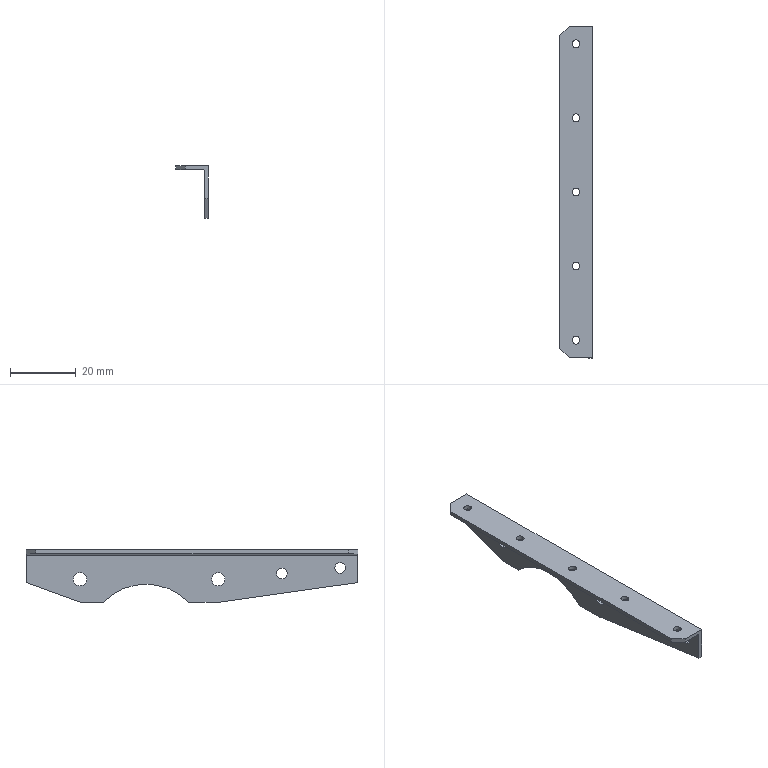Part | SolidWorks | features BaseBody 1 | 1 solid | 34 faces | box 10 x 100.8 x 16 mm | volume 2588 mm3 | cylinder 21 | plane 13 | commonest cylinder face diameters 2.4 x10 3.2 x4 4 x4 36 x2 1 x1
STEP:
#1=CARTESIAN_POINT('',(0.,5.4,-3.947));
#2=VERTEX_POINT('',#1);
#3=CARTESIAN_POINT('',(0.,5.4,-7.147));
#4=VERTEX_POINT('',#3);
#5=CARTESIAN_POINT('',(0.,5.4,-5.547));
#6=DIRECTION('',(1.,0.,0.));
#7=DIRECTION('',(0.,0.,1.));
#8=AXIS2_PLACEMENT_3D('',#5,#6,#7);
#9=CIRCLE('',#8,1.6);
#10=EDGE_CURVE('',#2,#4,#9,.T.);
#11=ORIENTED_EDGE('',*,*,#10,.T.);
#12=CARTESIAN_POINT('',(-1.2,5.4,-7.147));
#13=VERTEX_POINT('',#12);
#14=CARTESIAN_POINT('',(0.,5.4,-7.147));
#15=DIRECTION('',(-1.,0.,0.));
#16=VECTOR('',#15,1000.);
#17=LINE('',#14,#16);
#18=EDGE_CURVE('',#4,#13,#17,.T.);
#19=ORIENTED_EDGE('',*,*,#18,.T.);
#20=CARTESIAN_POINT('',(-1.2,5.4,-3.947));
#21=VERTEX_POINT('',#20);
#22=CARTESIAN_POINT('',(-1.2,5.4,-5.547));
#23=DIRECTION('',(-1.,0.,0.));
#24=DIRECTION('',(0.,0.,1.));
#25=AXIS2_PLACEMENT_3D('',#22,#23,#24);
#26=CIRCLE('',#25,1.6);
#27=EDGE_CURVE('',#13,#21,#26,.T.);
#28=ORIENTED_EDGE('',*,*,#27,.T.);
#29=CARTESIAN_POINT('',(0.,5.4,-3.947));
#30=DIRECTION('',(-1.,0.,0.));
#31=VECTOR('',#30,1000.);
#32=LINE('',#29,#31);
#33=EDGE_CURVE('',#2,#21,#32,.T.);
#34=ORIENTED_EDGE('',*,*,#33,.F.);
#35=EDGE_LOOP('',(#11,#19,#28,#34));
#36=FACE_OUTER_BOUND('',#35,.T.);
#37=CARTESIAN_POINT('',(0.,5.4,-5.547));
#38=DIRECTION('',(-1.,0.,0.));
#39=DIRECTION('',(0.,0.,1.));
#40=AXIS2_PLACEMENT_3D('',#37,#38,#39);
#41=CYLINDRICAL_SURFACE('',#40,1.6);
#42=ADVANCED_FACE('',(#36),#41,.F.);
#43=CARTESIAN_POINT('',(0.,84.4,-7.));
#44=VERTEX_POINT('',#43);
#45=CARTESIAN_POINT('',(0.,84.4,-11.));
#46=VERTEX_POINT('',#45);
#47=CARTESIAN_POINT('',(0.,84.4,-9.));
#48=DIRECTION('',(1.,0.,0.));
#49=DIRECTION('',(0.,0.,1.));
#50=AXIS2_PLACEMENT_3D('',#47,#48,#49);
#51=CIRCLE('',#50,2.);
#52=EDGE_CURVE('',#44,#46,#51,.T.);
#53=ORIENTED_EDGE('',*,*,#52,.T.);
#54=CARTESIAN_POINT('',(-1.2,84.4,-11.));
#55=VERTEX_POINT('',#54);
#56=CARTESIAN_POINT('',(0.,84.4,-11.));
#57=DIRECTION('',(-1.,0.,0.));
#58=VECTOR('',#57,1000.);
#59=LINE('',#56,#58);
#60=EDGE_CURVE('',#46,#55,#59,.T.);
#61=ORIENTED_EDGE('',*,*,#60,.T.);
#62=CARTESIAN_POINT('',(-1.2,84.4,-7.));
#63=VERTEX_POINT('',#62);
#64=CARTESIAN_POINT('',(-1.2,84.4,-9.));
#65=DIRECTION('',(-1.,0.,0.));
#66=DIRECTION('',(0.,0.,1.));
#67=AXIS2_PLACEMENT_3D('',#64,#65,#66);
#68=CIRCLE('',#67,2.);
#69=EDGE_CURVE('',#55,#63,#68,.T.);
#70=ORIENTED_EDGE('',*,*,#69,.T.);
#71=CARTESIAN_POINT('',(0.,84.4,-7.));
#72=DIRECTION('',(-1.,0.,0.));
#73=VECTOR('',#72,1000.);
#74=LINE('',#71,#73);
#75=EDGE_CURVE('',#44,#63,#74,.T.);
#76=ORIENTED_EDGE('',*,*,#75,.F.);
#77=EDGE_LOOP('',(#53,#61,#70,#76));
#78=FACE_OUTER_BOUND('',#77,.T.);
#79=CARTESIAN_POINT('',(0.,84.4,-9.));
#80=DIRECTION('',(-1.,0.,0.));
#81=DIRECTION('',(0.,0.,1.));
#82=AXIS2_PLACEMENT_3D('',#79,#80,#81);
#83=CYLINDRICAL_SURFACE('',#82,2.);
#84=ADVANCED_FACE('',(#78),#83,.F.);
#85=CARTESIAN_POINT('',(0.,42.4,-7.));
#86=VERTEX_POINT('',#85);
#87=CARTESIAN_POINT('',(0.,42.4,-11.));
#88=VERTEX_POINT('',#87);
#89=CARTESIAN_POINT('',(0.,42.4,-9.));
#90=DIRECTION('',(1.,0.,0.));
#91=DIRECTION('',(0.,0.,1.));
#92=AXIS2_PLACEMENT_3D('',#89,#90,#91);
#93=CIRCLE('',#92,2.);
#94=EDGE_CURVE('',#86,#88,#93,.T.);
#95=ORIENTED_EDGE('',*,*,#94,.T.);
#96=CARTESIAN_POINT('',(-1.2,42.4,-11.));
#97=VERTEX_POINT('',#96);
#98=CARTESIAN_POINT('',(0.,42.4,-11.));
#99=DIRECTION('',(-1.,0.,0.));
#100=VECTOR('',#99,1000.);
#101=LINE('',#98,#100);
#102=EDGE_CURVE('',#88,#97,#101,.T.);
#103=ORIENTED_EDGE('',*,*,#102,.T.);
#104=CARTESIAN_POINT('',(-1.2,42.4,-7.));
#105=VERTEX_POINT('',#104);
#106=CARTESIAN_POINT('',(-1.2,42.4,-9.));
#107=DIRECTION('',(-1.,0.,0.));
#108=DIRECTION('',(0.,0.,1.));
#109=AXIS2_PLACEMENT_3D('',#106,#107,#108);
#110=CIRCLE('',#109,2.);
#111=EDGE_CURVE('',#97,#105,#110,.T.);
#112=ORIENTED_EDGE('',*,*,#111,.T.);
#113=CARTESIAN_POINT('',(0.,42.4,-7.));
#114=DIRECTION('',(-1.,0.,0.));
#115=VECTOR('',#114,1000.);
#116=LINE('',#113,#115);
#117=EDGE_CURVE('',#86,#105,#116,.T.);
#118=ORIENTED_EDGE('',*,*,#117,.F.);
#119=EDGE_LOOP('',(#95,#103,#112,#118));
#120=FACE_OUTER_BOUND('',#119,.T.);
#121=CARTESIAN_POINT('',(0.,42.4,-9.));
#122=DIRECTION('',(-1.,0.,0.));
#123=DIRECTION('',(0.,0.,1.));
#124=AXIS2_PLACEMENT_3D('',#121,#122,#123);
#125=CYLINDRICAL_SURFACE('',#124,2.);
#126=ADVANCED_FACE('',(#120),#125,.F.);
#127=CARTESIAN_POINT('',(0.,23.103,-5.599));
#128=VERTEX_POINT('',#127);
#129=CARTESIAN_POINT('',(0.,23.103,-8.799));
#130=VERTEX_POINT('',#129);
#131=CARTESIAN_POINT('',(0.,23.103,-7.199));
#132=DIRECTION('',(1.,0.,0.));
#133=DIRECTION('',(0.,0.,1.));
#134=AXIS2_PLACEMENT_3D('',#131,#132,#133);
#135=CIRCLE('',#134,1.6);
#136=EDGE_CURVE('',#128,#130,#135,.T.);
#137=ORIENTED_EDGE('',*,*,#136,.T.);
#138=CARTESIAN_POINT('',(-1.2,23.103,-8.799));
#139=VERTEX_POINT('',#138);
#140=CARTESIAN_POINT('',(0.,23.103,-8.799));
#141=DIRECTION('',(-1.,0.,0.));
#142=VECTOR('',#141,1000.);
#143=LINE('',#140,#142);
#144=EDGE_CURVE('',#130,#139,#143,.T.);
#145=ORIENTED_EDGE('',*,*,#144,.T.);
#146=CARTESIAN_POINT('',(-1.2,23.103,-5.599));
#147=VERTEX_POINT('',#146);
#148=CARTESIAN_POINT('',(-1.2,23.103,-7.199));
#149=DIRECTION('',(-1.,0.,0.));
#150=DIRECTION('',(0.,0.,1.));
#151=AXIS2_PLACEMENT_3D('',#148,#149,#150);
#152=CIRCLE('',#151,1.6);
#153=EDGE_CURVE('',#139,#147,#152,.T.);
#154=ORIENTED_EDGE('',*,*,#153,.T.);
#155=CARTESIAN_POINT('',(0.,23.103,-5.599));
#156=DIRECTION('',(-1.,0.,0.));
#157=VECTOR('',#156,1000.);
#158=LINE('',#155,#157);
#159=EDGE_CURVE('',#128,#147,#158,.T.);
#160=ORIENTED_EDGE('',*,*,#159,.F.);
#161=EDGE_LOOP('',(#137,#145,#154,#160));
#162=FACE_OUTER_BOUND('',#161,.T.);
#163=CARTESIAN_POINT('',(0.,23.103,-7.199));
#164=DIRECTION('',(-1.,0.,0.));
#165=DIRECTION('',(0.,0.,1.));
#166=AXIS2_PLACEMENT_3D('',#163,#164,#165);
#167=CYLINDRICAL_SURFACE('',#166,1.6);
#168=ADVANCED_FACE('',(#162),#167,.F.);
#169=CARTESIAN_POINT('',(0.,77.352,-16.));
#170=VERTEX_POINT('',#169);
#171=CARTESIAN_POINT('',(0.,64.4,-10.5));
#172=VERTEX_POINT('',#171);
#173=CARTESIAN_POINT('',(0.,64.4,-28.5));
#174=DIRECTION('',(1.,0.,0.));
#175=DIRECTION('',(0.,0.,1.));
#176=AXIS2_PLACEMENT_3D('',#173,#174,#175);
#177=CIRCLE('',#176,18.);
#178=EDGE_CURVE('',#170,#172,#177,.T.);
#179=ORIENTED_EDGE('',*,*,#178,.T.);
#180=CARTESIAN_POINT('',(-1.2,64.4,-10.5));
#181=VERTEX_POINT('',#180);
#182=CARTESIAN_POINT('',(0.,64.4,-10.5));
#183=DIRECTION('',(-1.,0.,0.));
#184=VECTOR('',#183,1000.);
#185=LINE('',#182,#184);
#186=EDGE_CURVE('',#172,#181,#185,.T.);
#187=ORIENTED_EDGE('',*,*,#186,.T.);
#188=CARTESIAN_POINT('',(-1.2,77.352,-16.));
#189=VERTEX_POINT('',#188);
#190=CARTESIAN_POINT('',(-1.2,64.4,-28.5));
#191=DIRECTION('',(-1.,0.,0.));
#192=DIRECTION('',(0.,0.,1.));
#193=AXIS2_PLACEMENT_3D('',#190,#191,#192);
#194=CIRCLE('',#193,18.);
#195=EDGE_CURVE('',#181,#189,#194,.T.);
#196=ORIENTED_EDGE('',*,*,#195,.T.);
#197=CARTESIAN_POINT('',(-0.6,77.352,-16.));
#198=DIRECTION('',(1.,0.,0.));
#199=VECTOR('',#198,1000.);
#200=LINE('',#197,#199);
#201=EDGE_CURVE('',#189,#170,#200,.T.);
#202=ORIENTED_EDGE('',*,*,#201,.T.);
#203=EDGE_LOOP('',(#179,#187,#196,#202));
#204=FACE_OUTER_BOUND('',#203,.T.);
#205=CARTESIAN_POINT('',(0.,64.4,-28.5));
#206=DIRECTION('',(-1.,0.,0.));
#207=DIRECTION('',(0.,0.,1.));
#208=AXIS2_PLACEMENT_3D('',#205,#206,#207);
#209=CYLINDRICAL_SURFACE('',#208,18.);
#210=ADVANCED_FACE('',(#204),#209,.F.);
#211=CARTESIAN_POINT('',(-6.2,95.4,0.));
#212=VERTEX_POINT('',#211);
#213=CARTESIAN_POINT('',(-3.8,95.4,0.));
#214=VERTEX_POINT('',#213);
#215=CARTESIAN_POINT('',(-5.,95.4,0.));
#216=DIRECTION('',(0.,0.,1.));
#217=DIRECTION('',(-1.,0.,0.));
#218=AXIS2_PLACEMENT_3D('',#215,#216,#217);
#219=CIRCLE('',#218,1.2);
#220=EDGE_CURVE('',#212,#214,#219,.T.);
#221=ORIENTED_EDGE('',*,*,#220,.T.);
#222=CARTESIAN_POINT('',(-3.8,95.4,-1.2));
#223=VERTEX_POINT('',#222);
#224=CARTESIAN_POINT('',(-3.8,95.4,0.));
#225=DIRECTION('',(0.,0.,-1.));
#226=VECTOR('',#225,1000.);
#227=LINE('',#224,#226);
#228=EDGE_CURVE('',#214,#223,#227,.T.);
#229=ORIENTED_EDGE('',*,*,#228,.T.);
#230=CARTESIAN_POINT('',(-6.2,95.4,-1.2));
#231=VERTEX_POINT('',#230);
#232=CARTESIAN_POINT('',(-5.,95.4,-1.2));
#233=DIRECTION('',(0.,0.,-1.));
#234=DIRECTION('',(-1.,0.,0.));
#235=AXIS2_PLACEMENT_3D('',#232,#233,#234);
#236=CIRCLE('',#235,1.2);
#237=EDGE_CURVE('',#223,#231,#236,.T.);
#238=ORIENTED_EDGE('',*,*,#237,.T.);
#239=CARTESIAN_POINT('',(-6.2,95.4,0.));
#240=DIRECTION('',(0.,0.,-1.));
#241=VECTOR('',#240,1000.);
#242=LINE('',#239,#241);
#243=EDGE_CURVE('',#212,#231,#242,.T.);
#244=ORIENTED_EDGE('',*,*,#243,.F.);
#245=EDGE_LOOP('',(#221,#229,#238,#244));
#246=FACE_OUTER_BOUND('',#245,.T.);
#247=CARTESIAN_POINT('',(-5.,95.4,0.));
#248=DIRECTION('',(0.,0.,-1.));
#249=DIRECTION('',(-1.,0.,0.));
#250=AXIS2_PLACEMENT_3D('',#247,#248,#249);
#251=CYLINDRICAL_SURFACE('',#250,1.2);
#252=ADVANCED_FACE('',(#246),#251,.F.);
#253=CARTESIAN_POINT('',(-6.2,72.9,0.));
#254=VERTEX_POINT('',#253);
#255=CARTESIAN_POINT('',(-3.8,72.9,0.));
#256=VERTEX_POINT('',#255);
#257=CARTESIAN_POINT('',(-5.,72.9,0.));
#258=DIRECTION('',(0.,0.,1.));
#259=DIRECTION('',(-1.,0.,0.));
#260=AXIS2_PLACEMENT_3D('',#257,#258,#259);
#261=CIRCLE('',#260,1.2);
#262=EDGE_CURVE('',#254,#256,#261,.T.);
#263=ORIENTED_EDGE('',*,*,#262,.T.);
#264=CARTESIAN_POINT('',(-3.8,72.9,-1.2));
#265=VERTEX_POINT('',#264);
#266=CARTESIAN_POINT('',(-3.8,72.9,0.));
#267=DIRECTION('',(0.,0.,-1.));
#268=VECTOR('',#267,1000.);
#269=LINE('',#266,#268);
#270=EDGE_CURVE('',#256,#265,#269,.T.);
#271=ORIENTED_EDGE('',*,*,#270,.T.);
#272=CARTESIAN_POINT('',(-6.2,72.9,-1.2));
#273=VERTEX_POINT('',#272);
#274=CARTESIAN_POINT('',(-5.,72.9,-1.2));
#275=DIRECTION('',(0.,0.,-1.));
#276=DIRECTION('',(-1.,0.,0.));
#277=AXIS2_PLACEMENT_3D('',#274,#275,#276);
#278=CIRCLE('',#277,1.2);
#279=EDGE_CURVE('',#265,#273,#278,.T.);
#280=ORIENTED_EDGE('',*,*,#279,.T.);
#281=CARTESIAN_POINT('',(-6.2,72.9,0.));
#282=DIRECTION('',(0.,0.,-1.));
#283=VECTOR('',#282,1000.);
#284=LINE('',#281,#283);
#285=EDGE_CURVE('',#254,#273,#284,.T.);
#286=ORIENTED_EDGE('',*,*,#285,.F.);
#287=EDGE_LOOP('',(#263,#271,#280,#286));
#288=FACE_OUTER_BOUND('',#287,.T.);
#289=CARTESIAN_POINT('',(-5.,72.9,0.));
#290=DIRECTION('',(0.,0.,-1.));
#291=DIRECTION('',(-1.,0.,0.));
#292=AXIS2_PLACEMENT_3D('',#289,#290,#291);
#293=CYLINDRICAL_SURFACE('',#292,1.2);
#294=ADVANCED_FACE('',(#288),#293,.F.);
#295=CARTESIAN_POINT('',(-6.2,50.4,0.));
#296=VERTEX_POINT('',#295);
#297=CARTESIAN_POINT('',(-3.8,50.4,0.));
#298=VERTEX_POINT('',#297);
#299=CARTESIAN_POINT('',(-5.,50.4,0.));
#300=DIRECTION('',(0.,0.,1.));
#301=DIRECTION('',(-1.,0.,0.));
#302=AXIS2_PLACEMENT_3D('',#299,#300,#301);
#303=CIRCLE('',#302,1.2);
#304=EDGE_CURVE('',#296,#298,#303,.T.);
#305=ORIENTED_EDGE('',*,*,#304,.T.);
#306=CARTESIAN_POINT('',(-3.8,50.4,-1.2));
#307=VERTEX_POINT('',#306);
#308=CARTESIAN_POINT('',(-3.8,50.4,0.));
#309=DIRECTION('',(0.,0.,-1.));
#310=VECTOR('',#309,1000.);
#311=LINE('',#308,#310);
#312=EDGE_CURVE('',#298,#307,#311,.T.);
#313=ORIENTED_EDGE('',*,*,#312,.T.);
#314=CARTESIAN_POINT('',(-6.2,50.4,-1.2));
#315=VERTEX_POINT('',#314);
#316=CARTESIAN_POINT('',(-5.,50.4,-1.2));
#317=DIRECTION('',(0.,0.,-1.));
#318=DIRECTION('',(-1.,0.,0.));
#319=AXIS2_PLACEMENT_3D('',#316,#317,#318);
#320=CIRCLE('',#319,1.2);
#321=EDGE_CURVE('',#307,#315,#320,.T.);
#322=ORIENTED_EDGE('',*,*,#321,.T.);
#323=CARTESIAN_POINT('',(-6.2,50.4,0.));
#324=DIRECTION('',(0.,0.,-1.));
#325=VECTOR('',#324,1000.);
#326=LINE('',#323,#325);
#327=EDGE_CURVE('',#296,#315,#326,.T.);
#328=ORIENTED_EDGE('',*,*,#327,.F.);
#329=EDGE_LOOP('',(#305,#313,#322,#328));
#330=FACE_OUTER_BOUND('',#329,.T.);
#331=CARTESIAN_POINT('',(-5.,50.4,0.));
#332=DIRECTION('',(0.,0.,-1.));
#333=DIRECTION('',(-1.,0.,0.));
#334=AXIS2_PLACEMENT_3D('',#331,#332,#333);
#335=CYLINDRICAL_SURFACE('',#334,1.2);
#336=ADVANCED_FACE('',(#330),#335,.F.);
#337=CARTESIAN_POINT('',(-6.2,5.4,0.));
#338=VERTEX_POINT('',#337);
#339=CARTESIAN_POINT('',(-3.8,5.4,0.));
#340=VERTEX_POINT('',#339);
#341=CARTESIAN_POINT('',(-5.,5.4,0.));
#342=DIRECTION('',(0.,0.,1.));
#343=DIRECTION('',(-1.,0.,0.));
#344=AXIS2_PLACEMENT_3D('',#341,#342,#343);
#345=CIRCLE('',#344,1.2);
#346=EDGE_CURVE('',#338,#340,#345,.T.);
#347=ORIENTED_EDGE('',*,*,#346,.T.);
#348=CARTESIAN_POINT('',(-3.8,5.4,-1.2));
#349=VERTEX_POINT('',#348);
#350=CARTESIAN_POINT('',(-3.8,5.4,0.));
#351=DIRECTION('',(0.,0.,-1.));
#352=VECTOR('',#351,1000.);
#353=LINE('',#350,#352);
#354=EDGE_CURVE('',#340,#349,#353,.T.);
#355=ORIENTED_EDGE('',*,*,#354,.T.);
#356=CARTESIAN_POINT('',(-6.2,5.4,-1.2));
#357=VERTEX_POINT('',#356);
#358=CARTESIAN_POINT('',(-5.,5.4,-1.2));
#359=DIRECTION('',(0.,0.,-1.));
#360=DIRECTION('',(-1.,0.,0.));
#361=AXIS2_PLACEMENT_3D('',#358,#359,#360);
#362=CIRCLE('',#361,1.2);
#363=EDGE_CURVE('',#349,#357,#362,.T.);
#364=ORIENTED_EDGE('',*,*,#363,.T.);
#365=CARTESIAN_POINT('',(-6.2,5.4,0.));
#366=DIRECTION('',(0.,0.,-1.));
#367=VECTOR('',#366,1000.);
#368=LINE('',#365,#367);
#369=EDGE_CURVE('',#338,#357,#368,.T.);
#370=ORIENTED_EDGE('',*,*,#369,.F.);
#371=EDGE_LOOP('',(#347,#355,#364,#370));
#372=FACE_OUTER_BOUND('',#371,.T.);
#373=CARTESIAN_POINT('',(-5.,5.4,0.));
#374=DIRECTION('',(0.,0.,-1.));
#375=DIRECTION('',(-1.,0.,0.));
#376=AXIS2_PLACEMENT_3D('',#373,#374,#375);
#377=CYLINDRICAL_SURFACE('',#376,1.2);
#378=ADVANCED_FACE('',(#372),#377,.F.);
#379=CARTESIAN_POINT('',(-6.2,27.9,0.));
#380=VERTEX_POINT('',#379);
#381=CARTESIAN_POINT('',(-3.8,27.9,0.));
#382=VERTEX_POINT('',#381);
#383=CARTESIAN_POINT('',(-5.,27.9,0.));
#384=DIRECTION('',(0.,0.,1.));
#385=DIRECTION('',(-1.,0.,0.));
#386=AXIS2_PLACEMENT_3D('',#383,#384,#385);
#387=CIRCLE('',#386,1.2);
#388=EDGE_CURVE('',#380,#382,#387,.T.);
#389=ORIENTED_EDGE('',*,*,#388,.T.);
#390=CARTESIAN_POINT('',(-3.8,27.9,-1.2));
#391=VERTEX_POINT('',#390);
#392=CARTESIAN_POINT('',(-3.8,27.9,0.));
#393=DIRECTION('',(0.,0.,-1.));
#394=VECTOR('',#393,1000.);
#395=LINE('',#392,#394);
#396=EDGE_CURVE('',#382,#391,#395,.T.);
#397=ORIENTED_EDGE('',*,*,#396,.T.);
#398=CARTESIAN_POINT('',(-6.2,27.9,-1.2));
#399=VERTEX_POINT('',#398);
#400=CARTESIAN_POINT('',(-5.,27.9,-1.2));
#401=DIRECTION('',(0.,0.,-1.));
#402=DIRECTION('',(-1.,0.,0.));
#403=AXIS2_PLACEMENT_3D('',#400,#401,#402);
#404=CIRCLE('',#403,1.2);
#405=EDGE_CURVE('',#391,#399,#404,.T.);
#406=ORIENTED_EDGE('',*,*,#405,.T.);
#407=CARTESIAN_POINT('',(-6.2,27.9,0.));
#408=DIRECTION('',(0.,0.,-1.));
#409=VECTOR('',#408,1000.);
#410=LINE('',#407,#409);
#411=EDGE_CURVE('',#380,#399,#410,.T.);
#412=ORIENTED_EDGE('',*,*,#411,.F.);
#413=EDGE_LOOP('',(#389,#397,#406,#412));
#414=FACE_OUTER_BOUND('',#413,.T.);
#415=CARTESIAN_POINT('',(-5.,27.9,0.));
#416=DIRECTION('',(0.,0.,-1.));
#417=DIRECTION('',(-1.,0.,0.));
#418=AXIS2_PLACEMENT_3D('',#415,#416,#417);
#419=CYLINDRICAL_SURFACE('',#418,1.2);
#420=ADVANCED_FACE('',(#414),#419,.F.);
#421=ORIENTED_EDGE('',*,*,#18,.F.);
#422=CARTESIAN_POINT('',(0.,5.4,-5.547));
#423=DIRECTION('',(1.,0.,0.));
#424=DIRECTION('',(0.,0.,1.));
#425=AXIS2_PLACEMENT_3D('',#422,#423,#424);
#426=CIRCLE('',#425,1.6);
#427=EDGE_CURVE('',#4,#2,#426,.T.);
#428=ORIENTED_EDGE('',*,*,#427,.T.);
#429=ORIENTED_EDGE('',*,*,#33,.T.);
#430=CARTESIAN_POINT('',(-1.2,5.4,-5.547));
#431=DIRECTION('',(-1.,0.,0.));
#432=DIRECTION('',(0.,0.,1.));
#433=AXIS2_PLACEMENT_3D('',#430,#431,#432);
#434=CIRCLE('',#433,1.6);
#435=EDGE_CURVE('',#21,#13,#434,.T.);
#436=ORIENTED_EDGE('',*,*,#435,.T.);
#437=EDGE_LOOP('',(#421,#428,#429,#436));
#438=FACE_OUTER_BOUND('',#437,.T.);
#439=CARTESIAN_POINT('',(0.,5.4,-5.547));
#440=DIRECTION('',(-1.,0.,0.));
#441=DIRECTION('',(0.,0.,1.));
#442=AXIS2_PLACEMENT_3D('',#439,#440,#441);
#443=CYLINDRICAL_SURFACE('',#442,1.6);
#444=ADVANCED_FACE('',(#438),#443,.F.);
#445=CARTESIAN_POINT('',(-1.2,84.4,-9.));
#446=DIRECTION('',(-1.,0.,0.));
#447=DIRECTION('',(0.,0.,1.));
#448=AXIS2_PLACEMENT_3D('',#445,#446,#447);
#449=CIRCLE('',#448,2.);
#450=EDGE_CURVE('',#63,#55,#449,.T.);
#451=ORIENTED_EDGE('',*,*,#450,.F.);
#452=ORIENTED_EDGE('',*,*,#69,.F.);
#453=EDGE_LOOP('',(#451,#452));
#454=FACE_BOUND('',#453,.T.);
#455=CARTESIAN_POINT('',(-1.2,42.4,-9.));
#456=DIRECTION('',(-1.,0.,0.));
#457=DIRECTION('',(0.,0.,1.));
#458=AXIS2_PLACEMENT_3D('',#455,#456,#457);
#459=CIRCLE('',#458,2.);
#460=EDGE_CURVE('',#105,#97,#459,.T.);
#461=ORIENTED_EDGE('',*,*,#460,.F.);
#462=ORIENTED_EDGE('',*,*,#111,.F.);
#463=EDGE_LOOP('',(#461,#462));
#464=FACE_BOUND('',#463,.T.);
#465=CARTESIAN_POINT('',(-1.2,23.103,-7.199));
#466=DIRECTION('',(-1.,0.,0.));
#467=DIRECTION('',(0.,0.,1.));
#468=AXIS2_PLACEMENT_3D('',#465,#466,#467);
#469=CIRCLE('',#468,1.6);
#470=EDGE_CURVE('',#147,#139,#469,.T.);
#471=ORIENTED_EDGE('',*,*,#470,.F.);
#472=ORIENTED_EDGE('',*,*,#153,.F.);
#473=EDGE_LOOP('',(#471,#472));
#474=FACE_BOUND('',#473,.T.);
#475=ORIENTED_EDGE('',*,*,#435,.F.);
#476=ORIENTED_EDGE('',*,*,#27,.F.);
#477=EDGE_LOOP('',(#475,#476));
#478=FACE_BOUND('',#477,.T.);
#479=CARTESIAN_POINT('',(-1.2,100.8,-1.7));
#480=VERTEX_POINT('',#479);
#481=CARTESIAN_POINT('',(-1.2,0.,-1.7));
#482=VERTEX_POINT('',#481);
#483=CARTESIAN_POINT('',(-1.2,50.4,-1.7));
#484=DIRECTION('',(0.,-1.,0.));
#485=VECTOR('',#484,1000.);
#486=LINE('',#483,#485);
#487=EDGE_CURVE('',#480,#482,#486,.T.);
#488=ORIENTED_EDGE('',*,*,#487,.F.);
#489=CARTESIAN_POINT('',(-1.2,100.8,-10.));
#490=VERTEX_POINT('',#489);
#491=CARTESIAN_POINT('',(-1.2,100.8,-8.85));
#492=DIRECTION('',(0.,0.,1.));
#493=VECTOR('',#492,1000.);
#494=LINE('',#491,#493);
#495=EDGE_CURVE('',#490,#480,#494,.T.);
#496=ORIENTED_EDGE('',*,*,#495,.F.);
#497=CARTESIAN_POINT('',(-1.2,84.4,-16.));
#498=VERTEX_POINT('',#497);
#499=CARTESIAN_POINT('',(-1.2,84.4,-16.));
#500=DIRECTION('',(0.,0.9391,0.3436));
#501=VECTOR('',#500,1000.);
#502=LINE('',#499,#501);
#503=EDGE_CURVE('',#498,#490,#502,.T.);
#504=ORIENTED_EDGE('',*,*,#503,.F.);
#505=CARTESIAN_POINT('',(-1.2,50.4,-16.));
#506=DIRECTION('',(0.,1.,0.));
#507=VECTOR('',#506,1000.);
#508=LINE('',#505,#507);
#509=EDGE_CURVE('',#189,#498,#508,.T.);
#510=ORIENTED_EDGE('',*,*,#509,.F.);
#511=ORIENTED_EDGE('',*,*,#195,.F.);
#512=CARTESIAN_POINT('',(-1.2,51.448,-16.));
#513=VERTEX_POINT('',#512);
#514=CARTESIAN_POINT('',(-1.2,64.4,-28.5));
#515=DIRECTION('',(-1.,0.,0.));
#516=DIRECTION('',(0.,0.,1.));
#517=AXIS2_PLACEMENT_3D('',#514,#515,#516);
#518=CIRCLE('',#517,18.);
#519=EDGE_CURVE('',#513,#181,#518,.T.);
#520=ORIENTED_EDGE('',*,*,#519,.F.);
#521=CARTESIAN_POINT('',(-1.2,42.4,-16.));
#522=VERTEX_POINT('',#521);
#523=CARTESIAN_POINT('',(-1.2,50.4,-16.));
#524=DIRECTION('',(0.,1.,0.));
#525=VECTOR('',#524,1000.);
#526=LINE('',#523,#525);
#527=EDGE_CURVE('',#522,#513,#526,.T.);
#528=ORIENTED_EDGE('',*,*,#527,.F.);
#529=CARTESIAN_POINT('',(-1.2,0.,-10.));
#530=VERTEX_POINT('',#529);
#531=CARTESIAN_POINT('',(-1.2,0.,-10.));
#532=DIRECTION('',(0.,0.9901,-0.1401));
#533=VECTOR('',#532,1000.);
#534=LINE('',#531,#533);
#535=EDGE_CURVE('',#530,#522,#534,.T.);
#536=ORIENTED_EDGE('',*,*,#535,.F.);
#537=CARTESIAN_POINT('',(-1.2,0.,-8.85));
#538=DIRECTION('',(0.,0.,-1.));
#539=VECTOR('',#538,1000.);
#540=LINE('',#537,#539);
#541=EDGE_CURVE('',#482,#530,#540,.T.);
#542=ORIENTED_EDGE('',*,*,#541,.F.);
#543=EDGE_LOOP('',(#488,#496,#504,#510,#511,#520,#528,#536,#542));
#544=FACE_OUTER_BOUND('',#543,.T.);
#545=CARTESIAN_POINT('',(-1.2,100.8,-16.));
#546=DIRECTION('',(1.,0.,0.));
#547=DIRECTION('',(0.,0.,1.));
#548=AXIS2_PLACEMENT_3D('',#545,#546,#547);
#549=PLANE('',#548);
#550=ADVANCED_FACE('',(#454,#464,#474,#478,#544),#549,.F.);
#551=ORIENTED_EDGE('',*,*,#52,.F.);
#552=CARTESIAN_POINT('',(0.,84.4,-9.));
#553=DIRECTION('',(1.,0.,0.));
#554=DIRECTION('',(0.,0.,1.));
#555=AXIS2_PLACEMENT_3D('',#552,#553,#554);
#556=CIRCLE('',#555,2.);
#557=EDGE_CURVE('',#46,#44,#556,.T.);
#558=ORIENTED_EDGE('',*,*,#557,.F.);
#559=EDGE_LOOP('',(#551,#558));
#560=FACE_BOUND('',#559,.T.);
#561=ORIENTED_EDGE('',*,*,#94,.F.);
#562=CARTESIAN_POINT('',(0.,42.4,-9.));
#563=DIRECTION('',(1.,0.,0.));
#564=DIRECTION('',(0.,0.,1.));
#565=AXIS2_PLACEMENT_3D('',#562,#563,#564);
#566=CIRCLE('',#565,2.);
#567=EDGE_CURVE('',#88,#86,#566,.T.);
#568=ORIENTED_EDGE('',*,*,#567,.F.);
#569=EDGE_LOOP('',(#561,#568));
#570=FACE_BOUND('',#569,.T.);
#571=ORIENTED_EDGE('',*,*,#136,.F.);
#572=CARTESIAN_POINT('',(0.,23.103,-7.199));
#573=DIRECTION('',(1.,0.,0.));
#574=DIRECTION('',(0.,0.,1.));
#575=AXIS2_PLACEMENT_3D('',#572,#573,#574);
#576=CIRCLE('',#575,1.6);
#577=EDGE_CURVE('',#130,#128,#576,.T.);
#578=ORIENTED_EDGE('',*,*,#577,.F.);
#579=EDGE_LOOP('',(#571,#578));
#580=FACE_BOUND('',#579,.T.);
#581=ORIENTED_EDGE('',*,*,#10,.F.);
#582=ORIENTED_EDGE('',*,*,#427,.F.);
#583=EDGE_LOOP('',(#581,#582));
#584=FACE_BOUND('',#583,.T.);
#585=ORIENTED_EDGE('',*,*,#178,.F.);
#586=CARTESIAN_POINT('',(0.,84.4,-16.));
#587=VERTEX_POINT('',#586);
#588=CARTESIAN_POINT('',(0.,50.4,-16.));
#589=DIRECTION('',(0.,-1.,0.));
#590=VECTOR('',#589,1000.);
#591=LINE('',#588,#590);
#592=EDGE_CURVE('',#587,#170,#591,.T.);
#593=ORIENTED_EDGE('',*,*,#592,.F.);
#594=CARTESIAN_POINT('',(0.,100.8,-10.));
#595=VERTEX_POINT('',#594);
#596=CARTESIAN_POINT('',(0.,84.4,-16.));
#597=DIRECTION('',(0.,-0.9391,-0.3436));
#598=VECTOR('',#597,1000.);
#599=LINE('',#596,#598);
#600=EDGE_CURVE('',#595,#587,#599,.T.);
#601=ORIENTED_EDGE('',*,*,#600,.F.);
#602=CARTESIAN_POINT('',(0.,100.8,0.));
#603=VERTEX_POINT('',#602);
#604=CARTESIAN_POINT('',(0.,100.8,-8.));
#605=DIRECTION('',(0.,0.,-1.));
#606=VECTOR('',#605,1000.);
#607=LINE('',#604,#606);
#608=EDGE_CURVE('',#603,#595,#607,.T.);
#609=ORIENTED_EDGE('',*,*,#608,.F.);
#610=CARTESIAN_POINT('',(0.,0.,0.));
#611=VERTEX_POINT('',#610);
#612=CARTESIAN_POINT('',(0.,50.4,0.));
#613=DIRECTION('',(0.,1.,0.));
#614=VECTOR('',#613,1000.);
#615=LINE('',#612,#614);
#616=EDGE_CURVE('',#611,#603,#615,.T.);
#617=ORIENTED_EDGE('',*,*,#616,.F.);
#618=CARTESIAN_POINT('',(0.,0.,-10.));
#619=VERTEX_POINT('',#618);
#620=CARTESIAN_POINT('',(0.,0.,-8.));
#621=DIRECTION('',(0.,0.,1.));
#622=VECTOR('',#621,1000.);
#623=LINE('',#620,#622);
#624=EDGE_CURVE('',#619,#611,#623,.T.);
#625=ORIENTED_EDGE('',*,*,#624,.F.);
#626=CARTESIAN_POINT('',(0.,42.4,-16.));
#627=VERTEX_POINT('',#626);
#628=CARTESIAN_POINT('',(0.,0.,-10.));
#629=DIRECTION('',(0.,-0.9901,0.1401));
#630=VECTOR('',#629,1000.);
#631=LINE('',#628,#630);
#632=EDGE_CURVE('',#627,#619,#631,.T.);
#633=ORIENTED_EDGE('',*,*,#632,.F.);
#634=CARTESIAN_POINT('',(0.,51.448,-16.));
#635=VERTEX_POINT('',#634);
#636=CARTESIAN_POINT('',(0.,50.4,-16.));
#637=DIRECTION('',(0.,-1.,0.));
#638=VECTOR('',#637,1000.);
#639=LINE('',#636,#638);
#640=EDGE_CURVE('',#635,#627,#639,.T.);
#641=ORIENTED_EDGE('',*,*,#640,.F.);
#642=CARTESIAN_POINT('',(0.,64.4,-28.5));
#643=DIRECTION('',(1.,0.,0.));
#644=DIRECTION('',(0.,0.,1.));
#645=AXIS2_PLACEMENT_3D('',#642,#643,#644);
#646=CIRCLE('',#645,18.);
#647=EDGE_CURVE('',#172,#635,#646,.T.);
#648=ORIENTED_EDGE('',*,*,#647,.F.);
#649=EDGE_LOOP('',(#585,#593,#601,#609,#617,#625,#633,#641,#648));
#650=FACE_OUTER_BOUND('',#649,.T.);
#651=CARTESIAN_POINT('',(0.,100.8,0.));
#652=DIRECTION('',(-1.,0.,0.));
#653=DIRECTION('',(0.,0.,-1.));
#654=AXIS2_PLACEMENT_3D('',#651,#652,#653);
#655=PLANE('',#654);
#656=ADVANCED_FACE('',(#560,#570,#580,#584,#650),#655,.F.);
#657=ORIENTED_EDGE('',*,*,#60,.F.);
#658=ORIENTED_EDGE('',*,*,#557,.T.);
#659=ORIENTED_EDGE('',*,*,#75,.T.);
#660=ORIENTED_EDGE('',*,*,#450,.T.);
#661=EDGE_LOOP('',(#657,#658,#659,#660));
#662=FACE_OUTER_BOUND('',#661,.T.);
#663=CARTESIAN_POINT('',(0.,84.4,-9.));
#664=DIRECTION('',(-1.,0.,0.));
#665=DIRECTION('',(0.,0.,1.));
#666=AXIS2_PLACEMENT_3D('',#663,#664,#665);
#667=CYLINDRICAL_SURFACE('',#666,2.);
#668=ADVANCED_FACE('',(#662),#667,.F.);
#669=ORIENTED_EDGE('',*,*,#102,.F.);
#670=ORIENTED_EDGE('',*,*,#567,.T.);
#671=ORIENTED_EDGE('',*,*,#117,.T.);
#672=ORIENTED_EDGE('',*,*,#460,.T.);
#673=EDGE_LOOP('',(#669,#670,#671,#672));
#674=FACE_OUTER_BOUND('',#673,.T.);
#675=CARTESIAN_POINT('',(0.,42.4,-9.));
#676=DIRECTION('',(-1.,0.,0.));
#677=DIRECTION('',(0.,0.,1.));
#678=AXIS2_PLACEMENT_3D('',#675,#676,#677);
#679=CYLINDRICAL_SURFACE('',#678,2.);
#680=ADVANCED_FACE('',(#674),#679,.F.);
#681=ORIENTED_EDGE('',*,*,#144,.F.);
#682=ORIENTED_EDGE('',*,*,#577,.T.);
#683=ORIENTED_EDGE('',*,*,#159,.T.);
#684=ORIENTED_EDGE('',*,*,#470,.T.);
#685=EDGE_LOOP('',(#681,#682,#683,#684));
#686=FACE_OUTER_BOUND('',#685,.T.);
#687=CARTESIAN_POINT('',(0.,23.103,-7.199));
#688=DIRECTION('',(-1.,0.,0.));
#689=DIRECTION('',(0.,0.,1.));
#690=AXIS2_PLACEMENT_3D('',#687,#688,#689);
#691=CYLINDRICAL_SURFACE('',#690,1.6);
#692=ADVANCED_FACE('',(#686),#691,.F.);
#693=CARTESIAN_POINT('',(-7.,0.,0.));
#694=VERTEX_POINT('',#693);
#695=CARTESIAN_POINT('',(-3.5,0.,0.));
#696=DIRECTION('',(1.,0.,0.));
#697=VECTOR('',#696,1000.);
#698=LINE('',#695,#697);
#699=EDGE_CURVE('',#694,#611,#698,.T.);
#700=ORIENTED_EDGE('',*,*,#699,.F.);
#701=CARTESIAN_POINT('',(-7.,0.,-1.2));
#702=VERTEX_POINT('',#701);
#703=CARTESIAN_POINT('',(-7.,0.,-0.6));
#704=DIRECTION('',(0.,0.,-1.));
#705=VECTOR('',#704,1000.);
#706=LINE('',#703,#705);
#707=EDGE_CURVE('',#694,#702,#706,.T.);
#708=ORIENTED_EDGE('',*,*,#707,.T.);
#709=CARTESIAN_POINT('',(-1.7,0.,-1.2));
#710=VERTEX_POINT('',#709);
#711=CARTESIAN_POINT('',(-3.5,0.,-1.2));
#712=DIRECTION('',(-1.,0.,0.));
#713=VECTOR('',#712,1000.);
#714=LINE('',#711,#713);
#715=EDGE_CURVE('',#710,#702,#714,.T.);
#716=ORIENTED_EDGE('',*,*,#715,.F.);
#717=CARTESIAN_POINT('',(-1.7,0.,-1.7));
#718=DIRECTION('',(0.,-1.,0.));
#719=DIRECTION('',(0.,0.,-1.));
#720=AXIS2_PLACEMENT_3D('',#717,#718,#719);
#721=CIRCLE('',#720,0.5);
#722=EDGE_CURVE('',#482,#710,#721,.T.);
#723=ORIENTED_EDGE('',*,*,#722,.F.);
#724=ORIENTED_EDGE('',*,*,#541,.T.);
#725=CARTESIAN_POINT('',(-3.5,0.,-10.));
#726=DIRECTION('',(-1.,0.,0.));
#727=VECTOR('',#726,1000.);
#728=LINE('',#725,#727);
#729=EDGE_CURVE('',#619,#530,#728,.T.);
#730=ORIENTED_EDGE('',*,*,#729,.F.);
#731=ORIENTED_EDGE('',*,*,#624,.T.);
#732=EDGE_LOOP('',(#700,#708,#716,#723,#724,#730,#731));
#733=FACE_OUTER_BOUND('',#732,.T.);
#734=CARTESIAN_POINT('',(0.,0.,0.));
#735=DIRECTION('',(0.,1.,0.));
#736=DIRECTION('',(0.,0.,-1.));
#737=AXIS2_PLACEMENT_3D('',#734,#735,#736);
#738=PLANE('',#737);
#739=ADVANCED_FACE('',(#733),#738,.F.);
#740=CARTESIAN_POINT('',(-1.7,100.8,-1.2));
#741=VERTEX_POINT('',#740);
#742=CARTESIAN_POINT('',(-1.7,100.8,-1.7));
#743=DIRECTION('',(0.,1.,0.));
#744=DIRECTION('',(0.,0.,-1.));
#745=AXIS2_PLACEMENT_3D('',#742,#743,#744);
#746=CIRCLE('',#745,0.5);
#747=EDGE_CURVE('',#741,#480,#746,.T.);
#748=ORIENTED_EDGE('',*,*,#747,.T.);
#749=ORIENTED_EDGE('',*,*,#487,.T.);
#750=ORIENTED_EDGE('',*,*,#722,.T.);
#751=CARTESIAN_POINT('',(-1.7,50.4,-1.2));
#752=DIRECTION('',(0.,1.,0.));
#753=VECTOR('',#752,1000.);
#754=LINE('',#751,#753);
#755=EDGE_CURVE('',#710,#741,#754,.T.);
#756=ORIENTED_EDGE('',*,*,#755,.T.);
#757=EDGE_LOOP('',(#748,#749,#750,#756));
#758=FACE_OUTER_BOUND('',#757,.T.);
#759=CARTESIAN_POINT('',(-1.7,100.8,-1.7));
#760=DIRECTION('',(0.,-1.,0.));
#761=DIRECTION('',(0.,0.,-1.));
#762=AXIS2_PLACEMENT_3D('',#759,#760,#761);
#763=CYLINDRICAL_SURFACE('',#762,0.5);
#764=ADVANCED_FACE('',(#758),#763,.F.);
#765=CARTESIAN_POINT('',(-7.,100.8,0.));
#766=VERTEX_POINT('',#765);
#767=CARTESIAN_POINT('',(-3.5,100.8,0.));
#768=DIRECTION('',(1.,0.,0.));
#769=VECTOR('',#768,1000.);
#770=LINE('',#767,#769);
#771=EDGE_CURVE('',#766,#603,#770,.T.);
#772=ORIENTED_EDGE('',*,*,#771,.T.);
#773=ORIENTED_EDGE('',*,*,#608,.T.);
#774=CARTESIAN_POINT('',(-3.5,100.8,-10.));
#775=DIRECTION('',(-1.,0.,0.));
#776=VECTOR('',#775,1000.);
#777=LINE('',#774,#776);
#778=EDGE_CURVE('',#595,#490,#777,.T.);
#779=ORIENTED_EDGE('',*,*,#778,.T.);
#780=ORIENTED_EDGE('',*,*,#495,.T.);
#781=ORIENTED_EDGE('',*,*,#747,.F.);
#782=CARTESIAN_POINT('',(-7.,100.8,-1.2));
#783=VERTEX_POINT('',#782);
#784=CARTESIAN_POINT('',(-3.5,100.8,-1.2));
#785=DIRECTION('',(-1.,0.,0.));
#786=VECTOR('',#785,1000.);
#787=LINE('',#784,#786);
#788=EDGE_CURVE('',#741,#783,#787,.T.);
#789=ORIENTED_EDGE('',*,*,#788,.T.);
#790=CARTESIAN_POINT('',(-7.,100.8,-0.6));
#791=DIRECTION('',(0.,0.,-1.));
#792=VECTOR('',#791,1000.);
#793=LINE('',#790,#792);
#794=EDGE_CURVE('',#766,#783,#793,.T.);
#795=ORIENTED_EDGE('',*,*,#794,.F.);
#796=EDGE_LOOP('',(#772,#773,#779,#780,#781,#789,#795));
#797=FACE_OUTER_BOUND('',#796,.T.);
#798=CARTESIAN_POINT('',(0.,100.8,0.));
#799=DIRECTION('',(0.,1.,0.));
#800=DIRECTION('',(0.,0.,-1.));
#801=AXIS2_PLACEMENT_3D('',#798,#799,#800);
#802=PLANE('',#801);
#803=ADVANCED_FACE('',(#797),#802,.T.);
#804=ORIENTED_EDGE('',*,*,#600,.T.);
#805=CARTESIAN_POINT('',(-0.6,84.4,-16.));
#806=DIRECTION('',(1.,0.,0.));
#807=VECTOR('',#806,1000.);
#808=LINE('',#805,#807);
#809=EDGE_CURVE('',#498,#587,#808,.T.);
#810=ORIENTED_EDGE('',*,*,#809,.F.);
#811=ORIENTED_EDGE('',*,*,#503,.T.);
#812=ORIENTED_EDGE('',*,*,#778,.F.);
#813=EDGE_LOOP('',(#804,#810,#811,#812));
#814=FACE_OUTER_BOUND('',#813,.T.);
#815=CARTESIAN_POINT('',(0.,84.4,-16.));
#816=DIRECTION('',(0.,-0.3436,0.9391));
#817=DIRECTION('',(0.,0.9391,0.3436));
#818=AXIS2_PLACEMENT_3D('',#815,#816,#817);
#819=PLANE('',#818);
#820=ADVANCED_FACE('',(#814),#819,.F.);
#821=ORIENTED_EDGE('',*,*,#809,.T.);
#822=ORIENTED_EDGE('',*,*,#592,.T.);
#823=ORIENTED_EDGE('',*,*,#201,.F.);
#824=ORIENTED_EDGE('',*,*,#509,.T.);
#825=EDGE_LOOP('',(#821,#822,#823,#824));
#826=FACE_OUTER_BOUND('',#825,.T.);
#827=CARTESIAN_POINT('',(0.,84.4,-16.));
#828=DIRECTION('',(0.,0.,1.));
#829=DIRECTION('',(-1.,0.,0.));
#830=AXIS2_PLACEMENT_3D('',#827,#828,#829);
#831=PLANE('',#830);
#832=ADVANCED_FACE('',(#826),#831,.F.);
#833=ORIENTED_EDGE('',*,*,#186,.F.);
#834=ORIENTED_EDGE('',*,*,#647,.T.);
#835=CARTESIAN_POINT('',(-0.6,51.448,-16.));
#836=DIRECTION('',(-1.,0.,0.));
#837=VECTOR('',#836,1000.);
#838=LINE('',#835,#837);
#839=EDGE_CURVE('',#635,#513,#838,.T.);
#840=ORIENTED_EDGE('',*,*,#839,.T.);
#841=ORIENTED_EDGE('',*,*,#519,.T.);
#842=EDGE_LOOP('',(#833,#834,#840,#841));
#843=FACE_OUTER_BOUND('',#842,.T.);
#844=CARTESIAN_POINT('',(0.,64.4,-28.5));
#845=DIRECTION('',(-1.,0.,0.));
#846=DIRECTION('',(0.,0.,1.));
#847=AXIS2_PLACEMENT_3D('',#844,#845,#846);
#848=CYLINDRICAL_SURFACE('',#847,18.);
#849=ADVANCED_FACE('',(#843),#848,.F.);
#850=ORIENTED_EDGE('',*,*,#839,.F.);
#851=ORIENTED_EDGE('',*,*,#640,.T.);
#852=CARTESIAN_POINT('',(-0.6,42.4,-16.));
#853=DIRECTION('',(1.,0.,0.));
#854=VECTOR('',#853,1000.);
#855=LINE('',#852,#854);
#856=EDGE_CURVE('',#522,#627,#855,.T.);
#857=ORIENTED_EDGE('',*,*,#856,.F.);
#858=ORIENTED_EDGE('',*,*,#527,.T.);
#859=EDGE_LOOP('',(#850,#851,#857,#858));
#860=FACE_OUTER_BOUND('',#859,.T.);
#861=CARTESIAN_POINT('',(0.,51.448,-16.));
#862=DIRECTION('',(0.,0.,1.));
#863=DIRECTION('',(-1.,0.,0.));
#864=AXIS2_PLACEMENT_3D('',#861,#862,#863);
#865=PLANE('',#864);
#866=ADVANCED_FACE('',(#860),#865,.F.);
#867=ORIENTED_EDGE('',*,*,#632,.T.);
#868=ORIENTED_EDGE('',*,*,#729,.T.);
#869=ORIENTED_EDGE('',*,*,#535,.T.);
#870=ORIENTED_EDGE('',*,*,#856,.T.);
#871=EDGE_LOOP('',(#867,#868,#869,#870));
#872=FACE_OUTER_BOUND('',#871,.T.);
#873=CARTESIAN_POINT('',(0.,0.,-10.));
#874=DIRECTION('',(0.,0.1401,0.9901));
#875=DIRECTION('',(0.,0.9901,-0.1401));
#876=AXIS2_PLACEMENT_3D('',#873,#874,#875);
#877=PLANE('',#876);
#878=ADVANCED_FACE('',(#872),#877,.F.);
#879=ORIENTED_EDGE('',*,*,#220,.F.);
#880=CARTESIAN_POINT('',(-5.,95.4,0.));
#881=DIRECTION('',(0.,0.,1.));
#882=DIRECTION('',(-1.,0.,0.));
#883=AXIS2_PLACEMENT_3D('',#880,#881,#882);
#884=CIRCLE('',#883,1.2);
#885=EDGE_CURVE('',#214,#212,#884,.T.);
#886=ORIENTED_EDGE('',*,*,#885,.F.);
#887=EDGE_LOOP('',(#879,#886));
#888=FACE_BOUND('',#887,.T.);
#889=ORIENTED_EDGE('',*,*,#262,.F.);
#890=CARTESIAN_POINT('',(-5.,72.9,0.));
#891=DIRECTION('',(0.,0.,1.));
#892=DIRECTION('',(-1.,0.,0.));
#893=AXIS2_PLACEMENT_3D('',#890,#891,#892);
#894=CIRCLE('',#893,1.2);
#895=EDGE_CURVE('',#256,#254,#894,.T.);
#896=ORIENTED_EDGE('',*,*,#895,.F.);
#897=EDGE_LOOP('',(#889,#896));
#898=FACE_BOUND('',#897,.T.);
#899=ORIENTED_EDGE('',*,*,#304,.F.);
#900=CARTESIAN_POINT('',(-5.,50.4,0.));
#901=DIRECTION('',(0.,0.,1.));
#902=DIRECTION('',(-1.,0.,0.));
#903=AXIS2_PLACEMENT_3D('',#900,#901,#902);
#904=CIRCLE('',#903,1.2);
#905=EDGE_CURVE('',#298,#296,#904,.T.);
#906=ORIENTED_EDGE('',*,*,#905,.F.);
#907=EDGE_LOOP('',(#899,#906));
#908=FACE_BOUND('',#907,.T.);
#909=ORIENTED_EDGE('',*,*,#346,.F.);
#910=CARTESIAN_POINT('',(-5.,5.4,0.));
#911=DIRECTION('',(0.,0.,1.));
#912=DIRECTION('',(-1.,0.,0.));
#913=AXIS2_PLACEMENT_3D('',#910,#911,#912);
#914=CIRCLE('',#913,1.2);
#915=EDGE_CURVE('',#340,#338,#914,.T.);
#916=ORIENTED_EDGE('',*,*,#915,.F.);
#917=EDGE_LOOP('',(#909,#916));
#918=FACE_BOUND('',#917,.T.);
#919=ORIENTED_EDGE('',*,*,#388,.F.);
#920=CARTESIAN_POINT('',(-5.,27.9,0.));
#921=DIRECTION('',(0.,0.,1.));
#922=DIRECTION('',(-1.,0.,0.));
#923=AXIS2_PLACEMENT_3D('',#920,#921,#922);
#924=CIRCLE('',#923,1.2);
#925=EDGE_CURVE('',#382,#380,#924,.T.);
#926=ORIENTED_EDGE('',*,*,#925,.F.);
#927=EDGE_LOOP('',(#919,#926));
#928=FACE_BOUND('',#927,.T.);
#929=ORIENTED_EDGE('',*,*,#616,.T.);
#930=ORIENTED_EDGE('',*,*,#771,.F.);
#931=CARTESIAN_POINT('',(-10.,97.8,0.));
#932=VERTEX_POINT('',#931);
#933=CARTESIAN_POINT('',(-7.,100.8,0.));
#934=DIRECTION('',(0.7071,0.7071,0.));
#935=VECTOR('',#934,1000.);
#936=LINE('',#933,#935);
#937=EDGE_CURVE('',#932,#766,#936,.T.);
#938=ORIENTED_EDGE('',*,*,#937,.F.);
#939=CARTESIAN_POINT('',(-10.,3.,0.));
#940=VERTEX_POINT('',#939);
#941=CARTESIAN_POINT('',(-10.,50.4,0.));
#942=DIRECTION('',(0.,1.,0.));
#943=VECTOR('',#942,1000.);
#944=LINE('',#941,#943);
#945=EDGE_CURVE('',#940,#932,#944,.T.);
#946=ORIENTED_EDGE('',*,*,#945,.F.);
#947=CARTESIAN_POINT('',(-7.,0.,0.));
#948=DIRECTION('',(-0.7071,0.7071,0.));
#949=VECTOR('',#948,1000.);
#950=LINE('',#947,#949);
#951=EDGE_CURVE('',#694,#940,#950,.T.);
#952=ORIENTED_EDGE('',*,*,#951,.F.);
#953=ORIENTED_EDGE('',*,*,#699,.T.);
#954=EDGE_LOOP('',(#929,#930,#938,#946,#952,#953));
#955=FACE_OUTER_BOUND('',#954,.T.);
#956=CARTESIAN_POINT('',(-10.,100.8,0.));
#957=DIRECTION('',(0.,0.,-1.));
#958=DIRECTION('',(1.,0.,0.));
#959=AXIS2_PLACEMENT_3D('',#956,#957,#958);
#960=PLANE('',#959);
#961=ADVANCED_FACE('',(#888,#898,#908,#918,#928,#955),#960,.F.);
#962=CARTESIAN_POINT('',(-5.,95.4,-1.2));
#963=DIRECTION('',(0.,0.,-1.));
#964=DIRECTION('',(-1.,0.,0.));
#965=AXIS2_PLACEMENT_3D('',#962,#963,#964);
#966=CIRCLE('',#965,1.2);
#967=EDGE_CURVE('',#231,#223,#966,.T.);
#968=ORIENTED_EDGE('',*,*,#967,.F.);
#969=ORIENTED_EDGE('',*,*,#237,.F.);
#970=EDGE_LOOP('',(#968,#969));
#971=FACE_BOUND('',#970,.T.);
#972=CARTESIAN_POINT('',(-5.,72.9,-1.2));
#973=DIRECTION('',(0.,0.,-1.));
#974=DIRECTION('',(-1.,0.,0.));
#975=AXIS2_PLACEMENT_3D('',#972,#973,#974);
#976=CIRCLE('',#975,1.2);
#977=EDGE_CURVE('',#273,#265,#976,.T.);
#978=ORIENTED_EDGE('',*,*,#977,.F.);
#979=ORIENTED_EDGE('',*,*,#279,.F.);
#980=EDGE_LOOP('',(#978,#979));
#981=FACE_BOUND('',#980,.T.);
#982=CARTESIAN_POINT('',(-5.,50.4,-1.2));
#983=DIRECTION('',(0.,0.,-1.));
#984=DIRECTION('',(-1.,0.,0.));
#985=AXIS2_PLACEMENT_3D('',#982,#983,#984);
#986=CIRCLE('',#985,1.2);
#987=EDGE_CURVE('',#315,#307,#986,.T.);
#988=ORIENTED_EDGE('',*,*,#987,.F.);
#989=ORIENTED_EDGE('',*,*,#321,.F.);
#990=EDGE_LOOP('',(#988,#989));
#991=FACE_BOUND('',#990,.T.);
#992=CARTESIAN_POINT('',(-5.,5.4,-1.2));
#993=DIRECTION('',(0.,0.,-1.));
#994=DIRECTION('',(-1.,0.,0.));
#995=AXIS2_PLACEMENT_3D('',#992,#993,#994);
#996=CIRCLE('',#995,1.2);
#997=EDGE_CURVE('',#357,#349,#996,.T.);
#998=ORIENTED_EDGE('',*,*,#997,.F.);
#999=ORIENTED_EDGE('',*,*,#363,.F.);
#1000=EDGE_LOOP('',(#998,#999));
#1001=FACE_BOUND('',#1000,.T.);
#1002=CARTESIAN_POINT('',(-5.,27.9,-1.2));
#1003=DIRECTION('',(0.,0.,-1.));
#1004=DIRECTION('',(-1.,0.,0.));
#1005=AXIS2_PLACEMENT_3D('',#1002,#1003,#1004);
#1006=CIRCLE('',#1005,1.2);
#1007=EDGE_CURVE('',#399,#391,#1006,.T.);
#1008=ORIENTED_EDGE('',*,*,#1007,.F.);
#1009=ORIENTED_EDGE('',*,*,#405,.F.);
#1010=EDGE_LOOP('',(#1008,#1009));
#1011=FACE_BOUND('',#1010,.T.);
#1012=CARTESIAN_POINT('',(-10.,97.8,-1.2));
#1013=VERTEX_POINT('',#1012);
#1014=CARTESIAN_POINT('',(-7.,100.8,-1.2));
#1015=DIRECTION('',(-0.7071,-0.7071,0.));
#1016=VECTOR('',#1015,1000.);
#1017=LINE('',#1014,#1016);
#1018=EDGE_CURVE('',#783,#1013,#1017,.T.);
#1019=ORIENTED_EDGE('',*,*,#1018,.F.);
#1020=ORIENTED_EDGE('',*,*,#788,.F.);
#1021=ORIENTED_EDGE('',*,*,#755,.F.);
#1022=ORIENTED_EDGE('',*,*,#715,.T.);
#1023=CARTESIAN_POINT('',(-10.,3.,-1.2));
#1024=VERTEX_POINT('',#1023);
#1025=CARTESIAN_POINT('',(-7.,0.,-1.2));
#1026=DIRECTION('',(0.7071,-0.7071,0.));
#1027=VECTOR('',#1026,1000.);
#1028=LINE('',#1025,#1027);
#1029=EDGE_CURVE('',#1024,#702,#1028,.T.);
#1030=ORIENTED_EDGE('',*,*,#1029,.F.);
#1031=CARTESIAN_POINT('',(-10.,50.4,-1.2));
#1032=DIRECTION('',(0.,-1.,0.));
#1033=VECTOR('',#1032,1000.);
#1034=LINE('',#1031,#1033);
#1035=EDGE_CURVE('',#1013,#1024,#1034,.T.);
#1036=ORIENTED_EDGE('',*,*,#1035,.F.);
#1037=EDGE_LOOP('',(#1019,#1020,#1021,#1022,#1030,#1036));
#1038=FACE_OUTER_BOUND('',#1037,.T.);
#1039=CARTESIAN_POINT('',(-1.7,100.8,-1.2));
#1040=DIRECTION('',(0.,0.,1.));
#1041=DIRECTION('',(-1.,0.,0.));
#1042=AXIS2_PLACEMENT_3D('',#1039,#1040,#1041);
#1043=PLANE('',#1042);
#1044=ADVANCED_FACE('',(#971,#981,#991,#1001,#1011,#1038),#1043,.F.);
#1045=ORIENTED_EDGE('',*,*,#228,.F.);
#1046=ORIENTED_EDGE('',*,*,#885,.T.);
#1047=ORIENTED_EDGE('',*,*,#243,.T.);
#1048=ORIENTED_EDGE('',*,*,#967,.T.);
#1049=EDGE_LOOP('',(#1045,#1046,#1047,#1048));
#1050=FACE_OUTER_BOUND('',#1049,.T.);
#1051=CARTESIAN_POINT('',(-5.,95.4,0.));
#1052=DIRECTION('',(0.,0.,-1.));
#1053=DIRECTION('',(-1.,0.,0.));
#1054=AXIS2_PLACEMENT_3D('',#1051,#1052,#1053);
#1055=CYLINDRICAL_SURFACE('',#1054,1.2);
#1056=ADVANCED_FACE('',(#1050),#1055,.F.);
#1057=ORIENTED_EDGE('',*,*,#270,.F.);
#1058=ORIENTED_EDGE('',*,*,#895,.T.);
#1059=ORIENTED_EDGE('',*,*,#285,.T.);
#1060=ORIENTED_EDGE('',*,*,#977,.T.);
#1061=EDGE_LOOP('',(#1057,#1058,#1059,#1060));
#1062=FACE_OUTER_BOUND('',#1061,.T.);
#1063=CARTESIAN_POINT('',(-5.,72.9,0.));
#1064=DIRECTION('',(0.,0.,-1.));
#1065=DIRECTION('',(-1.,0.,0.));
#1066=AXIS2_PLACEMENT_3D('',#1063,#1064,#1065);
#1067=CYLINDRICAL_SURFACE('',#1066,1.2);
#1068=ADVANCED_FACE('',(#1062),#1067,.F.);
#1069=ORIENTED_EDGE('',*,*,#312,.F.);
#1070=ORIENTED_EDGE('',*,*,#905,.T.);
#1071=ORIENTED_EDGE('',*,*,#327,.T.);
#1072=ORIENTED_EDGE('',*,*,#987,.T.);
#1073=EDGE_LOOP('',(#1069,#1070,#1071,#1072));
#1074=FACE_OUTER_BOUND('',#1073,.T.);
#1075=CARTESIAN_POINT('',(-5.,50.4,0.));
#1076=DIRECTION('',(0.,0.,-1.));
#1077=DIRECTION('',(-1.,0.,0.));
#1078=AXIS2_PLACEMENT_3D('',#1075,#1076,#1077);
#1079=CYLINDRICAL_SURFACE('',#1078,1.2);
#1080=ADVANCED_FACE('',(#1074),#1079,.F.);
#1081=ORIENTED_EDGE('',*,*,#354,.F.);
#1082=ORIENTED_EDGE('',*,*,#915,.T.);
#1083=ORIENTED_EDGE('',*,*,#369,.T.);
#1084=ORIENTED_EDGE('',*,*,#997,.T.);
#1085=EDGE_LOOP('',(#1081,#1082,#1083,#1084));
#1086=FACE_OUTER_BOUND('',#1085,.T.);
#1087=CARTESIAN_POINT('',(-5.,5.4,0.));
#1088=DIRECTION('',(0.,0.,-1.));
#1089=DIRECTION('',(-1.,0.,0.));
#1090=AXIS2_PLACEMENT_3D('',#1087,#1088,#1089);
#1091=CYLINDRICAL_SURFACE('',#1090,1.2);
#1092=ADVANCED_FACE('',(#1086),#1091,.F.);
#1093=ORIENTED_EDGE('',*,*,#396,.F.);
#1094=ORIENTED_EDGE('',*,*,#925,.T.);
#1095=ORIENTED_EDGE('',*,*,#411,.T.);
#1096=ORIENTED_EDGE('',*,*,#1007,.T.);
#1097=EDGE_LOOP('',(#1093,#1094,#1095,#1096));
#1098=FACE_OUTER_BOUND('',#1097,.T.);
#1099=CARTESIAN_POINT('',(-5.,27.9,0.));
#1100=DIRECTION('',(0.,0.,-1.));
#1101=DIRECTION('',(-1.,0.,0.));
#1102=AXIS2_PLACEMENT_3D('',#1099,#1100,#1101);
#1103=CYLINDRICAL_SURFACE('',#1102,1.2);
#1104=ADVANCED_FACE('',(#1098),#1103,.F.);
#1105=ORIENTED_EDGE('',*,*,#1018,.T.);
#1106=CARTESIAN_POINT('',(-10.,97.8,-0.6));
#1107=DIRECTION('',(0.,0.,1.));
#1108=VECTOR('',#1107,1000.);
#1109=LINE('',#1106,#1108);
#1110=EDGE_CURVE('',#1013,#932,#1109,.T.);
#1111=ORIENTED_EDGE('',*,*,#1110,.T.);
#1112=ORIENTED_EDGE('',*,*,#937,.T.);
#1113=ORIENTED_EDGE('',*,*,#794,.T.);
#1114=EDGE_LOOP('',(#1105,#1111,#1112,#1113));
#1115=FACE_OUTER_BOUND('',#1114,.T.);
#1116=CARTESIAN_POINT('',(-7.,100.8,-1.2));
#1117=DIRECTION('',(-0.7071,0.7071,0.));
#1118=DIRECTION('',(-0.7071,-0.7071,0.));
#1119=AXIS2_PLACEMENT_3D('',#1116,#1117,#1118);
#1120=PLANE('',#1119);
#1121=ADVANCED_FACE('',(#1115),#1120,.T.);
#1122=ORIENTED_EDGE('',*,*,#1110,.F.);
#1123=ORIENTED_EDGE('',*,*,#1035,.T.);
#1124=CARTESIAN_POINT('',(-10.,3.,-0.6));
#1125=DIRECTION('',(0.,0.,-1.));
#1126=VECTOR('',#1125,1000.);
#1127=LINE('',#1124,#1126);
#1128=EDGE_CURVE('',#940,#1024,#1127,.T.);
#1129=ORIENTED_EDGE('',*,*,#1128,.F.);
#1130=ORIENTED_EDGE('',*,*,#945,.T.);
#1131=EDGE_LOOP('',(#1122,#1123,#1129,#1130));
#1132=FACE_OUTER_BOUND('',#1131,.T.);
#1133=CARTESIAN_POINT('',(-10.,97.8,-1.2));
#1134=DIRECTION('',(1.,0.,0.));
#1135=DIRECTION('',(0.,0.,1.));
#1136=AXIS2_PLACEMENT_3D('',#1133,#1134,#1135);
#1137=PLANE('',#1136);
#1138=ADVANCED_FACE('',(#1132),#1137,.F.);
#1139=ORIENTED_EDGE('',*,*,#1128,.T.);
#1140=ORIENTED_EDGE('',*,*,#1029,.T.);
#1141=ORIENTED_EDGE('',*,*,#707,.F.);
#1142=ORIENTED_EDGE('',*,*,#951,.T.);
#1143=EDGE_LOOP('',(#1139,#1140,#1141,#1142));
#1144=FACE_OUTER_BOUND('',#1143,.T.);
#1145=CARTESIAN_POINT('',(-7.,0.,-1.2));
#1146=DIRECTION('',(0.7071,0.7071,0.));
#1147=DIRECTION('',(-0.7071,0.7071,0.));
#1148=AXIS2_PLACEMENT_3D('',#1145,#1146,#1147);
#1149=PLANE('',#1148);
#1150=ADVANCED_FACE('',(#1144),#1149,.F.);
#1151=CLOSED_SHELL('',(#42,#84,#126,#168,#210,#252,#294,#336,#378,#420,#444,#550,#656,#668,#680,#692,#739,#764,#803,#820,#832,#849,#866,#878,#961,#1044,#1056,#1068,#1080,#1092,#1104,#1121,#1138,#1150));
#1152=MANIFOLD_SOLID_BREP('',#1151);
#1153=CARTESIAN_POINT('',(0.,0.,0.));
#1154=DIRECTION('',(0.,0.,1.));
#1155=DIRECTION('',(1.,0.,0.));
#1156=AXIS2_PLACEMENT_3D('',#1153,#1154,#1155);
#1157=(LENGTH_UNIT()NAMED_UNIT(*)SI_UNIT(.MILLI.,.METRE.));
#1158=UNCERTAINTY_MEASURE_WITH_UNIT(LENGTH_MEASURE(0.00001),#1157,'','');
#1159=(NAMED_UNIT(*)PLANE_ANGLE_UNIT()SI_UNIT($,.RADIAN.));
#1160=(NAMED_UNIT(*)SI_UNIT($,.STERADIAN.)SOLID_ANGLE_UNIT());
#1161=(GEOMETRIC_REPRESENTATION_CONTEXT(3)GLOBAL_UNCERTAINTY_ASSIGNED_CONTEXT((#1158))GLOBAL_UNIT_ASSIGNED_CONTEXT((#1157,#1159,#1160))REPRESENTATION_CONTEXT('',''));
#1162=ADVANCED_BREP_SHAPE_REPRESENTATION('',(#1152,#1156),#1161);